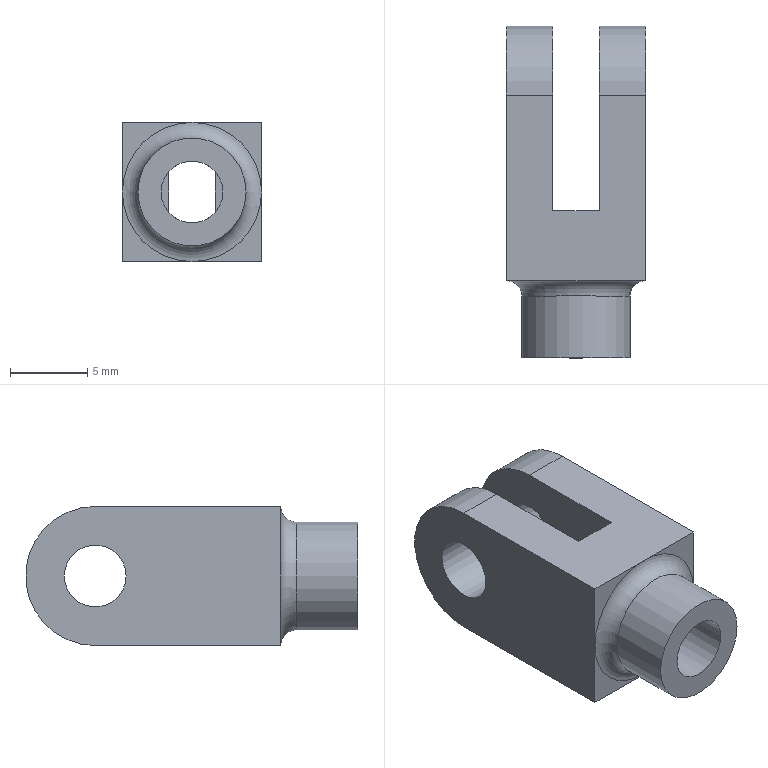Part | STEP file | 2-11.3 | 1 solid | 22 faces | box 9 x 21.5 x 9 mm | volume 963.016 mm3 | plane 15 | cylinder 6 | torus 1 | commonest cylinder face diameters 4 x3 9 x2 7 x1